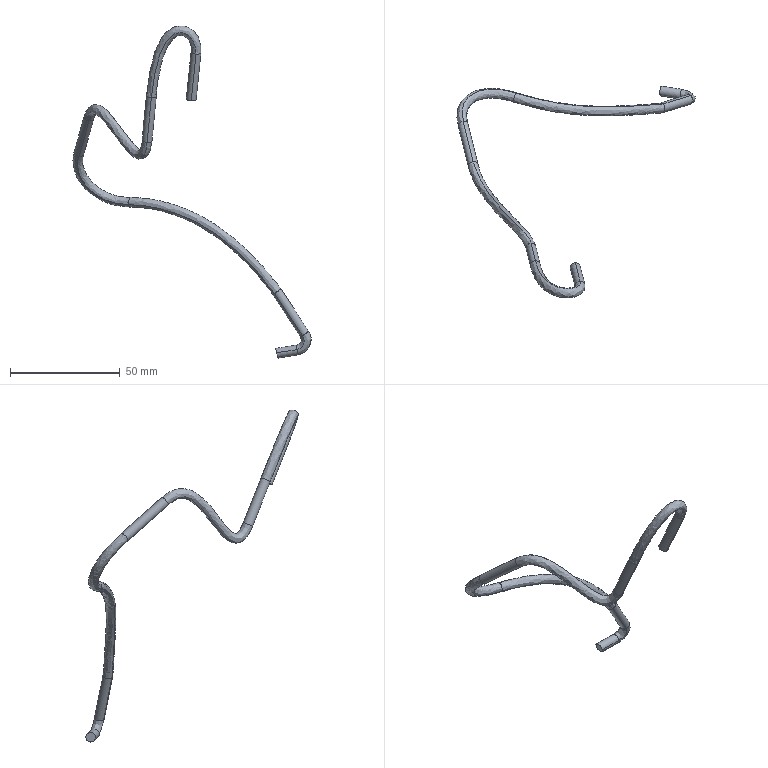Part | STEP file | PN_0031 | 1 solid | 22 faces | box 108.679 x 96.834 x 151.567 mm | volume 5490 mm3 | spline 14 | cylinder 6 | plane 2 | commonest cylinder face diameters 4.5 x6